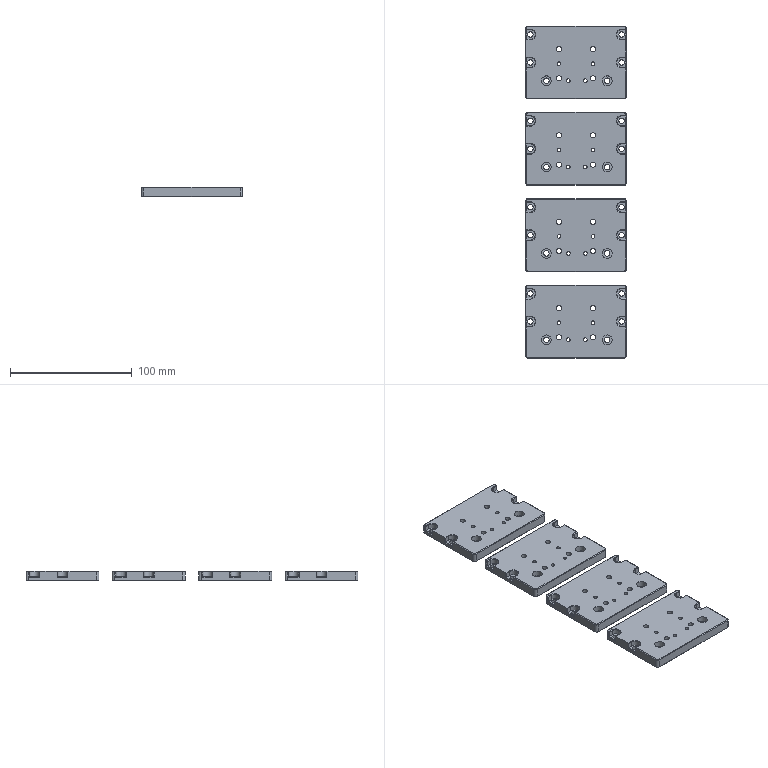Part | 4 solids | 372 faces | box 83 x 273 x 8 mm | volume 148886 mm3 | plane 228 | cylinder 96 | cone 48 | commonest cylinder face diameters 4.5 x24 8 x24 3 x16 4 x16 4.2 x16